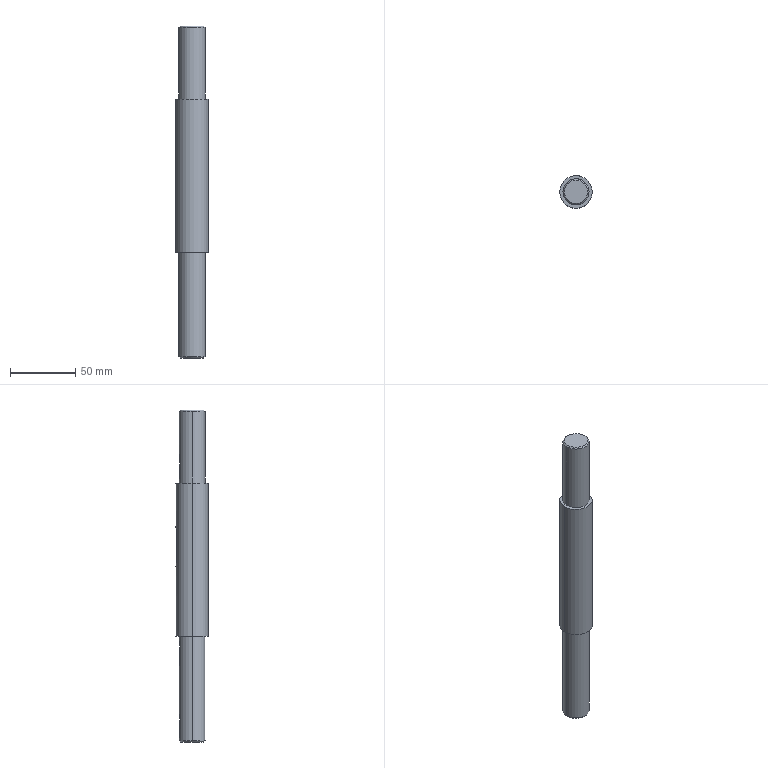Part | SolidWorks | features BaseBody 1 | 1 solid | 42 faces | box 25 x 25 x 254.5 mm | volume 96928 mm3 | cylinder 20 | plane 16 | cone 6 | commonest cylinder face diameters 6 x9 20 x4 8 x3 8.5 x2 25 x2